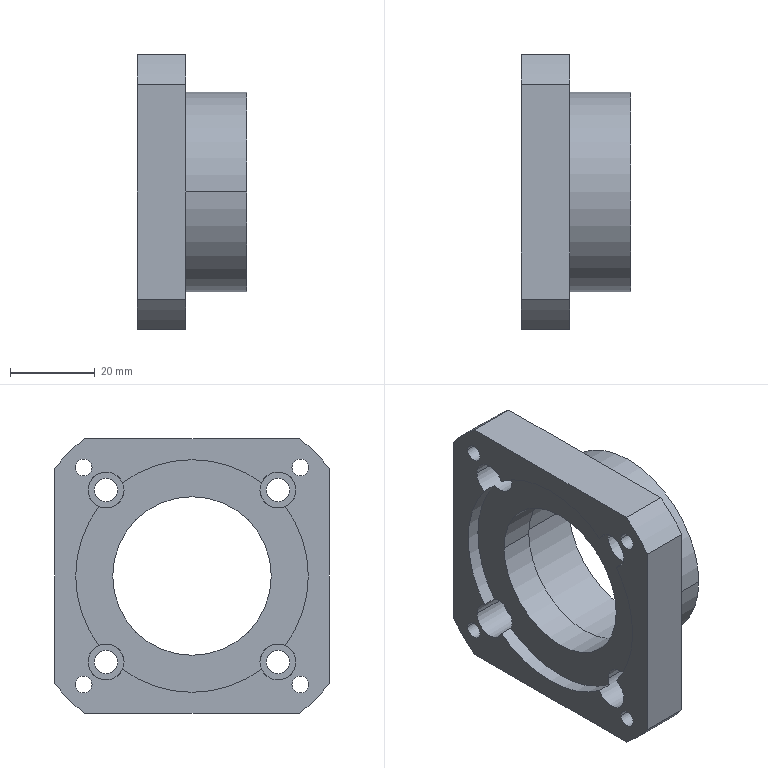Part | STEP file | 2026.6.15-Main Assembly图.sldasm-Part-110 | 1 solid | 52 faces | box 26 x 65 x 65 mm | volume 35291 mm3 | cylinder 39 | plane 13 | commonest cylinder face diameters 4 x8 5.5 x8 8.5 x8 55 x5 82.5 x4 37.5 x2